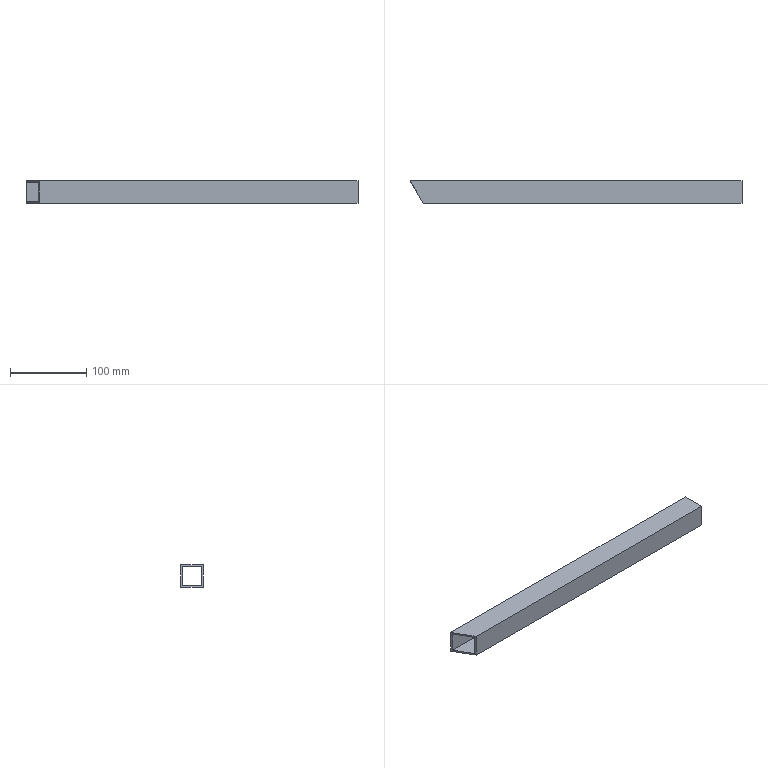Part | NX | features solid 2 | 1 solid | 10 faces | box 434.378 x 30 x 30 mm | volume 95361 mm3 | plane 10
STEP:
#1=CARTESIAN_POINT('',(380.,330.,-45.));
#2=VERTEX_POINT('',#1);
#3=CARTESIAN_POINT('',(380.,330.,-15.));
#4=VERTEX_POINT('',#3);
#5=CARTESIAN_POINT('',(380.,330.,-45.));
#6=DIRECTION('',(0.,0.,-1.));
#7=VECTOR('',#6,1000.);
#8=LINE('',#5,#7);
#9=EDGE_CURVE('',#2,#4,#8,.F.);
#10=ORIENTED_EDGE('',*,*,#9,.F.);
#11=CARTESIAN_POINT('',(-54.378,330.,-45.));
#12=VERTEX_POINT('',#11);
#13=CARTESIAN_POINT('',(25.,330.,-45.));
#14=DIRECTION('',(1.,0.,0.));
#15=VECTOR('',#14,1000.);
#16=LINE('',#13,#15);
#17=EDGE_CURVE('',#12,#2,#16,.T.);
#18=ORIENTED_EDGE('',*,*,#17,.F.);
#19=CARTESIAN_POINT('',(-54.378,330.,-15.));
#20=VERTEX_POINT('',#19);
#21=CARTESIAN_POINT('',(-54.378,330.,-75.));
#22=DIRECTION('',(0.,0.,-1.));
#23=VECTOR('',#22,1000.);
#24=LINE('',#21,#23);
#25=EDGE_CURVE('',#12,#20,#24,.F.);
#26=ORIENTED_EDGE('',*,*,#25,.T.);
#27=CARTESIAN_POINT('',(25.,330.,-15.));
#28=DIRECTION('',(1.,0.,0.));
#29=VECTOR('',#28,1000.);
#30=LINE('',#27,#29);
#31=EDGE_CURVE('',#20,#4,#30,.T.);
#32=ORIENTED_EDGE('',*,*,#31,.T.);
#33=EDGE_LOOP('',(#10,#18,#26,#32));
#34=FACE_BOUND('',#33,.T.);
#35=CARTESIAN_POINT('',(25.,330.,-45.));
#36=DIRECTION('',(0.,-1.,0.));
#37=DIRECTION('',(1.,0.,0.));
#38=AXIS2_PLACEMENT_3D('',#35,#36,#37);
#39=PLANE('',#38);
#40=ADVANCED_FACE('',(#34),#39,.F.);
#41=CARTESIAN_POINT('',(380.,300.,-15.));
#42=VERTEX_POINT('',#41);
#43=CARTESIAN_POINT('',(380.,300.,-45.));
#44=VERTEX_POINT('',#43);
#45=CARTESIAN_POINT('',(380.,300.,-45.));
#46=DIRECTION('',(0.,0.,-1.));
#47=VECTOR('',#46,1000.);
#48=LINE('',#45,#47);
#49=EDGE_CURVE('',#42,#44,#48,.T.);
#50=ORIENTED_EDGE('',*,*,#49,.F.);
#51=CARTESIAN_POINT('',(-37.058,300.,-15.));
#52=VERTEX_POINT('',#51);
#53=CARTESIAN_POINT('',(25.,300.,-15.));
#54=DIRECTION('',(1.,0.,0.));
#55=VECTOR('',#54,1000.);
#56=LINE('',#53,#55);
#57=EDGE_CURVE('',#52,#42,#56,.T.);
#58=ORIENTED_EDGE('',*,*,#57,.F.);
#59=CARTESIAN_POINT('',(-37.058,300.,-45.));
#60=VERTEX_POINT('',#59);
#61=CARTESIAN_POINT('',(-37.058,300.,-75.));
#62=DIRECTION('',(0.,0.,-1.));
#63=VECTOR('',#62,1000.);
#64=LINE('',#61,#63);
#65=EDGE_CURVE('',#52,#60,#64,.T.);
#66=ORIENTED_EDGE('',*,*,#65,.T.);
#67=CARTESIAN_POINT('',(25.,300.,-45.));
#68=DIRECTION('',(1.,0.,0.));
#69=VECTOR('',#68,1000.);
#70=LINE('',#67,#69);
#71=EDGE_CURVE('',#60,#44,#70,.T.);
#72=ORIENTED_EDGE('',*,*,#71,.T.);
#73=EDGE_LOOP('',(#50,#58,#66,#72));
#74=FACE_BOUND('',#73,.T.);
#75=CARTESIAN_POINT('',(25.,300.,-45.));
#76=DIRECTION('',(0.,-1.,0.));
#77=DIRECTION('',(1.,0.,0.));
#78=AXIS2_PLACEMENT_3D('',#75,#76,#77);
#79=PLANE('',#78);
#80=ADVANCED_FACE('',(#74),#79,.T.);
#81=CARTESIAN_POINT('',(-53.224,328.,-43.));
#82=VERTEX_POINT('',#81);
#83=CARTESIAN_POINT('',(380.,328.,-43.));
#84=VERTEX_POINT('',#83);
#85=CARTESIAN_POINT('',(25.,328.,-43.));
#86=DIRECTION('',(-1.,0.,0.));
#87=VECTOR('',#86,1000.);
#88=LINE('',#85,#87);
#89=EDGE_CURVE('',#82,#84,#88,.F.);
#90=ORIENTED_EDGE('',*,*,#89,.T.);
#91=CARTESIAN_POINT('',(380.,328.,-17.));
#92=VERTEX_POINT('',#91);
#93=CARTESIAN_POINT('',(380.,328.,-45.));
#94=DIRECTION('',(0.,0.,-1.));
#95=VECTOR('',#94,1000.);
#96=LINE('',#93,#95);
#97=EDGE_CURVE('',#84,#92,#96,.F.);
#98=ORIENTED_EDGE('',*,*,#97,.T.);
#99=CARTESIAN_POINT('',(-53.224,328.,-17.));
#100=VERTEX_POINT('',#99);
#101=CARTESIAN_POINT('',(25.,328.,-17.));
#102=DIRECTION('',(-1.,0.,0.));
#103=VECTOR('',#102,1000.);
#104=LINE('',#101,#103);
#105=EDGE_CURVE('',#100,#92,#104,.F.);
#106=ORIENTED_EDGE('',*,*,#105,.F.);
#107=CARTESIAN_POINT('',(-53.224,328.,-75.));
#108=DIRECTION('',(0.,0.,-1.));
#109=VECTOR('',#108,1000.);
#110=LINE('',#107,#109);
#111=EDGE_CURVE('',#82,#100,#110,.F.);
#112=ORIENTED_EDGE('',*,*,#111,.F.);
#113=EDGE_LOOP('',(#90,#98,#106,#112));
#114=FACE_BOUND('',#113,.T.);
#115=CARTESIAN_POINT('',(25.,328.,-45.));
#116=DIRECTION('',(0.,-1.,0.));
#117=DIRECTION('',(1.,0.,0.));
#118=AXIS2_PLACEMENT_3D('',#115,#116,#117);
#119=PLANE('',#118);
#120=ADVANCED_FACE('',(#114),#119,.T.);
#121=CARTESIAN_POINT('',(-38.212,302.,-17.));
#122=VERTEX_POINT('',#121);
#123=CARTESIAN_POINT('',(380.,302.,-17.));
#124=VERTEX_POINT('',#123);
#125=CARTESIAN_POINT('',(25.,302.,-17.));
#126=DIRECTION('',(1.,0.,0.));
#127=VECTOR('',#126,1000.);
#128=LINE('',#125,#127);
#129=EDGE_CURVE('',#122,#124,#128,.T.);
#130=ORIENTED_EDGE('',*,*,#129,.T.);
#131=CARTESIAN_POINT('',(380.,302.,-43.));
#132=VERTEX_POINT('',#131);
#133=CARTESIAN_POINT('',(380.,302.,-45.));
#134=DIRECTION('',(0.,0.,-1.));
#135=VECTOR('',#134,1000.);
#136=LINE('',#133,#135);
#137=EDGE_CURVE('',#124,#132,#136,.T.);
#138=ORIENTED_EDGE('',*,*,#137,.T.);
#139=CARTESIAN_POINT('',(-38.212,302.,-43.));
#140=VERTEX_POINT('',#139);
#141=CARTESIAN_POINT('',(25.,302.,-43.));
#142=DIRECTION('',(1.,0.,0.));
#143=VECTOR('',#142,1000.);
#144=LINE('',#141,#143);
#145=EDGE_CURVE('',#140,#132,#144,.T.);
#146=ORIENTED_EDGE('',*,*,#145,.F.);
#147=CARTESIAN_POINT('',(-38.212,302.,-75.));
#148=DIRECTION('',(0.,0.,-1.));
#149=VECTOR('',#148,1000.);
#150=LINE('',#147,#149);
#151=EDGE_CURVE('',#122,#140,#150,.T.);
#152=ORIENTED_EDGE('',*,*,#151,.F.);
#153=EDGE_LOOP('',(#130,#138,#146,#152));
#154=FACE_BOUND('',#153,.T.);
#155=CARTESIAN_POINT('',(25.,302.,-45.));
#156=DIRECTION('',(0.,-1.,0.));
#157=DIRECTION('',(1.,0.,0.));
#158=AXIS2_PLACEMENT_3D('',#155,#156,#157);
#159=PLANE('',#158);
#160=ADVANCED_FACE('',(#154),#159,.F.);
#161=CARTESIAN_POINT('',(380.,300.,-15.));
#162=DIRECTION('',(0.,-1.,0.));
#163=VECTOR('',#162,1000.);
#164=LINE('',#161,#163);
#165=EDGE_CURVE('',#4,#42,#164,.T.);
#166=ORIENTED_EDGE('',*,*,#165,.F.);
#167=ORIENTED_EDGE('',*,*,#31,.F.);
#168=CARTESIAN_POINT('',(-115.,435.,-15.));
#169=DIRECTION('',(0.5,-0.866,0.));
#170=VECTOR('',#169,1000.);
#171=LINE('',#168,#170);
#172=EDGE_CURVE('',#20,#52,#171,.T.);
#173=ORIENTED_EDGE('',*,*,#172,.T.);
#174=ORIENTED_EDGE('',*,*,#57,.T.);
#175=EDGE_LOOP('',(#166,#167,#173,#174));
#176=FACE_BOUND('',#175,.T.);
#177=CARTESIAN_POINT('',(25.,300.,-15.));
#178=DIRECTION('',(0.,0.,1.));
#179=DIRECTION('',(1.,0.,0.));
#180=AXIS2_PLACEMENT_3D('',#177,#178,#179);
#181=PLANE('',#180);
#182=ADVANCED_FACE('',(#176),#181,.T.);
#183=ORIENTED_EDGE('',*,*,#17,.T.);
#184=CARTESIAN_POINT('',(380.,300.,-45.));
#185=DIRECTION('',(0.,-1.,0.));
#186=VECTOR('',#185,1000.);
#187=LINE('',#184,#186);
#188=EDGE_CURVE('',#2,#44,#187,.T.);
#189=ORIENTED_EDGE('',*,*,#188,.T.);
#190=ORIENTED_EDGE('',*,*,#71,.F.);
#191=CARTESIAN_POINT('',(-21.543,273.128,-45.));
#192=DIRECTION('',(-0.5,0.866,0.));
#193=VECTOR('',#192,1000.);
#194=LINE('',#191,#193);
#195=EDGE_CURVE('',#60,#12,#194,.T.);
#196=ORIENTED_EDGE('',*,*,#195,.T.);
#197=EDGE_LOOP('',(#183,#189,#190,#196));
#198=FACE_BOUND('',#197,.T.);
#199=CARTESIAN_POINT('',(25.,300.,-45.));
#200=DIRECTION('',(0.,0.,1.));
#201=DIRECTION('',(1.,0.,0.));
#202=AXIS2_PLACEMENT_3D('',#199,#200,#201);
#203=PLANE('',#202);
#204=ADVANCED_FACE('',(#198),#203,.F.);
#205=ORIENTED_EDGE('',*,*,#105,.T.);
#206=CARTESIAN_POINT('',(380.,300.,-17.));
#207=DIRECTION('',(0.,-1.,0.));
#208=VECTOR('',#207,1000.);
#209=LINE('',#206,#208);
#210=EDGE_CURVE('',#92,#124,#209,.T.);
#211=ORIENTED_EDGE('',*,*,#210,.T.);
#212=ORIENTED_EDGE('',*,*,#129,.F.);
#213=CARTESIAN_POINT('',(-115.,435.,-17.));
#214=DIRECTION('',(0.5,-0.866,0.));
#215=VECTOR('',#214,1000.);
#216=LINE('',#213,#215);
#217=EDGE_CURVE('',#100,#122,#216,.T.);
#218=ORIENTED_EDGE('',*,*,#217,.F.);
#219=EDGE_LOOP('',(#205,#211,#212,#218));
#220=FACE_BOUND('',#219,.T.);
#221=CARTESIAN_POINT('',(25.,300.,-17.));
#222=DIRECTION('',(0.,0.,1.));
#223=DIRECTION('',(1.,0.,0.));
#224=AXIS2_PLACEMENT_3D('',#221,#222,#223);
#225=PLANE('',#224);
#226=ADVANCED_FACE('',(#220),#225,.F.);
#227=CARTESIAN_POINT('',(380.,300.,-43.));
#228=DIRECTION('',(0.,-1.,0.));
#229=VECTOR('',#228,1000.);
#230=LINE('',#227,#229);
#231=EDGE_CURVE('',#84,#132,#230,.T.);
#232=ORIENTED_EDGE('',*,*,#231,.F.);
#233=ORIENTED_EDGE('',*,*,#89,.F.);
#234=CARTESIAN_POINT('',(-21.543,273.128,-43.));
#235=DIRECTION('',(-0.5,0.866,0.));
#236=VECTOR('',#235,1000.);
#237=LINE('',#234,#236);
#238=EDGE_CURVE('',#140,#82,#237,.T.);
#239=ORIENTED_EDGE('',*,*,#238,.F.);
#240=ORIENTED_EDGE('',*,*,#145,.T.);
#241=EDGE_LOOP('',(#232,#233,#239,#240));
#242=FACE_BOUND('',#241,.T.);
#243=CARTESIAN_POINT('',(25.,300.,-43.));
#244=DIRECTION('',(0.,0.,1.));
#245=DIRECTION('',(1.,0.,0.));
#246=AXIS2_PLACEMENT_3D('',#243,#244,#245);
#247=PLANE('',#246);
#248=ADVANCED_FACE('',(#242),#247,.T.);
#249=ORIENTED_EDGE('',*,*,#25,.F.);
#250=ORIENTED_EDGE('',*,*,#195,.F.);
#251=ORIENTED_EDGE('',*,*,#65,.F.);
#252=ORIENTED_EDGE('',*,*,#172,.F.);
#253=EDGE_LOOP('',(#249,#250,#251,#252));
#254=FACE_BOUND('',#253,.T.);
#255=ORIENTED_EDGE('',*,*,#238,.T.);
#256=ORIENTED_EDGE('',*,*,#111,.T.);
#257=ORIENTED_EDGE('',*,*,#217,.T.);
#258=ORIENTED_EDGE('',*,*,#151,.T.);
#259=EDGE_LOOP('',(#255,#256,#257,#258));
#260=FACE_BOUND('',#259,.T.);
#261=CARTESIAN_POINT('',(-115.,435.,-75.));
#262=DIRECTION('',(0.866,0.5,0.));
#263=DIRECTION('',(0.,0.,1.));
#264=AXIS2_PLACEMENT_3D('',#261,#262,#263);
#265=PLANE('',#264);
#266=ADVANCED_FACE('',(#254,#260),#265,.F.);
#267=ORIENTED_EDGE('',*,*,#165,.T.);
#268=ORIENTED_EDGE('',*,*,#49,.T.);
#269=ORIENTED_EDGE('',*,*,#188,.F.);
#270=ORIENTED_EDGE('',*,*,#9,.T.);
#271=EDGE_LOOP('',(#267,#268,#269,#270));
#272=FACE_BOUND('',#271,.T.);
#273=ORIENTED_EDGE('',*,*,#97,.F.);
#274=ORIENTED_EDGE('',*,*,#231,.T.);
#275=ORIENTED_EDGE('',*,*,#137,.F.);
#276=ORIENTED_EDGE('',*,*,#210,.F.);
#277=EDGE_LOOP('',(#273,#274,#275,#276));
#278=FACE_BOUND('',#277,.T.);
#279=CARTESIAN_POINT('',(380.,335.,-125.));
#280=DIRECTION('',(-1.,0.,0.));
#281=DIRECTION('',(0.,0.,1.));
#282=AXIS2_PLACEMENT_3D('',#279,#280,#281);
#283=PLANE('',#282);
#284=ADVANCED_FACE('',(#272,#278),#283,.F.);
#285=CLOSED_SHELL('',(#40,#80,#120,#160,#182,#204,#226,#248,#266,#284));
#286=MANIFOLD_SOLID_BREP('',#285);
#287=(LENGTH_UNIT()NAMED_UNIT(*)SI_UNIT(.MILLI.,.METRE.));
#288=UNCERTAINTY_MEASURE_WITH_UNIT(LENGTH_MEASURE(0.00001),#287,'','');
#289=(NAMED_UNIT(*)PLANE_ANGLE_UNIT()SI_UNIT($,.RADIAN.));
#290=(NAMED_UNIT(*)SI_UNIT($,.STERADIAN.)SOLID_ANGLE_UNIT());
#291=(GEOMETRIC_REPRESENTATION_CONTEXT(3)GLOBAL_UNCERTAINTY_ASSIGNED_CONTEXT((#288))GLOBAL_UNIT_ASSIGNED_CONTEXT((#287,#289,#290))REPRESENTATION_CONTEXT('',''));
#292=ADVANCED_BREP_SHAPE_REPRESENTATION('',(#286),#291);